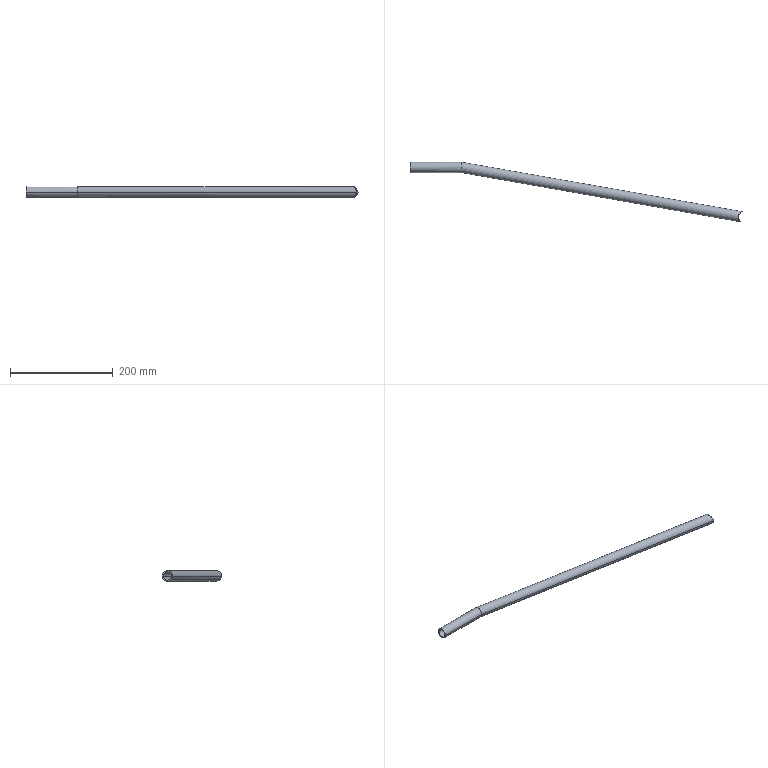Part | SolidWorks | features Cut 1, Sweep 1 | 1 solid | 10 faces | box 645.85 x 115.746 x 20 mm | volume 73442 mm3 | cylinder 9 | plane 1 | commonest cylinder face diameters 16 x4 20 x4 25 x1
STEP:
#1=CARTESIAN_POINT('',(-8.07,9.546,0.));
#2=VERTEX_POINT('',#1);
#3=CARTESIAN_POINT('',(-10.848,-6.211,0.));
#4=VERTEX_POINT('',#3);
#5=CARTESIAN_POINT('',(-8.07,9.546,0.));
#6=CARTESIAN_POINT('',(-8.07,9.546,-0.5418));
#7=CARTESIAN_POINT('',(-8.124,9.501,-1.074));
#8=CARTESIAN_POINT('',(-8.279,9.365,-1.86));
#9=CARTESIAN_POINT('',(-8.343,9.309,-2.12));
#10=CARTESIAN_POINT('',(-8.489,9.176,-2.623));
#11=CARTESIAN_POINT('',(-8.571,9.099,-2.869));
#12=CARTESIAN_POINT('',(-8.842,8.84,-3.586));
#13=CARTESIAN_POINT('',(-9.054,8.625,-4.044));
#14=CARTESIAN_POINT('',(-9.503,8.127,-4.888));
#15=CARTESIAN_POINT('',(-9.742,7.843,-5.28));
#16=CARTESIAN_POINT('',(-10.229,7.196,-6.005));
#17=CARTESIAN_POINT('',(-10.472,6.841,-6.33));
#18=CARTESIAN_POINT('',(-10.822,6.26,-6.76));
#19=CARTESIAN_POINT('',(-10.937,6.058,-6.894));
#20=CARTESIAN_POINT('',(-11.16,5.635,-7.143));
#21=CARTESIAN_POINT('',(-11.269,5.414,-7.258));
#22=CARTESIAN_POINT('',(-11.582,4.728,-7.568));
#23=CARTESIAN_POINT('',(-11.768,4.249,-7.727));
#24=CARTESIAN_POINT('',(-12.005,3.493,-7.889));
#25=CARTESIAN_POINT('',(-12.078,3.233,-7.931));
#26=CARTESIAN_POINT('',(-12.206,2.708,-7.986));
#27=CARTESIAN_POINT('',(-12.262,2.444,-8.));
#28=CARTESIAN_POINT('',(-12.355,1.915,-8.));
#29=CARTESIAN_POINT('',(-12.394,1.65,-7.987));
#30=CARTESIAN_POINT('',(-12.453,1.116,-7.934));
#31=CARTESIAN_POINT('',(-12.474,0.8473,-7.893));
#32=CARTESIAN_POINT('',(-12.511,0.04928,-7.732));
#33=CARTESIAN_POINT('',(-12.501,-0.4657,-7.574));
#34=CARTESIAN_POINT('',(-12.443,-1.214,-7.267));
#35=CARTESIAN_POINT('',(-12.417,-1.461,-7.152));
#36=CARTESIAN_POINT('',(-12.351,-1.938,-6.902));
#37=CARTESIAN_POINT('',(-12.313,-2.169,-6.768));
#38=CARTESIAN_POINT('',(-12.225,-2.616,-6.48));
#39=CARTESIAN_POINT('',(-12.177,-2.832,-6.326));
#40=CARTESIAN_POINT('',(-12.072,-3.251,-6.));
#41=CARTESIAN_POINT('',(-12.015,-3.454,-5.827));
#42=CARTESIAN_POINT('',(-11.838,-4.033,-5.285));
#43=CARTESIAN_POINT('',(-11.712,-4.381,-4.895));
#44=CARTESIAN_POINT('',(-11.46,-5.003,-4.052));
#45=CARTESIAN_POINT('',(-11.334,-5.278,-3.594));
#46=CARTESIAN_POINT('',(-11.113,-5.727,-2.638));
#47=CARTESIAN_POINT('',(-11.019,-5.904,-2.139));
#48=CARTESIAN_POINT('',(-10.885,-6.148,-1.085));
#49=CARTESIAN_POINT('',(-10.848,-6.211,-0.5447));
#50=CARTESIAN_POINT('',(-10.848,-6.211,0.));
#51=B_SPLINE_CURVE_WITH_KNOTS('',3,(#5,#6,#7,#8,#9,#10,#11,#12,#13,#14,#15,#16,#17,#18,#19,#20,#21,#22,#23,#24,#25,#26,#27,#28,#29,#30,#31,#32,#33,#34,#35,#36,#37,#38,#39,#40,#41,#42,#43,#44,#45,#46,#47,#48,#49,#50),.UNSPECIFIED.,.F.,.F.,(4,2,2,2,2,2,2,2,2,2,2,2,2,2,2,2,2,2,2,2,2,2,4),(0.02576,0.02737,0.02817,0.02897,0.03058,0.03218,0.03379,0.03459,0.03539,0.037,0.0378,0.0386,0.0394,0.04021,0.04181,0.04262,0.04342,0.04422,0.04502,0.04663,0.04823,0.04984,0.05144),.UNSPECIFIED.);
#52=EDGE_CURVE('',#2,#4,#51,.T.);
#53=ORIENTED_EDGE('',*,*,#52,.F.);
#54=CARTESIAN_POINT('',(-550.549,105.2,0.));
#55=VERTEX_POINT('',#54);
#56=CARTESIAN_POINT('',(1.389,7.878,0.));
#57=DIRECTION('',(-0.9848,0.1736,0.));
#58=VECTOR('',#57,1000.);
#59=LINE('',#56,#58);
#60=EDGE_CURVE('',#2,#55,#59,.T.);
#61=ORIENTED_EDGE('',*,*,#60,.T.);
#62=CARTESIAN_POINT('',(-551.949,89.2,0.));
#63=VERTEX_POINT('',#62);
#64=CARTESIAN_POINT('',(-550.549,105.2,0.));
#65=CARTESIAN_POINT('',(-550.549,105.2,-16.));
#66=CARTESIAN_POINT('',(-551.949,89.2,-16.));
#67=CARTESIAN_POINT('',(-551.949,89.2,0.));
#68=(BOUNDED_CURVE()B_SPLINE_CURVE(3,(#64,#65,#66,#67),.UNSPECIFIED.,.F.,.T.)B_SPLINE_CURVE_WITH_KNOTS((4,4),(3.142,6.283),.UNSPECIFIED.)CURVE()GEOMETRIC_REPRESENTATION_ITEM()RATIONAL_B_SPLINE_CURVE((1.,0.3333,0.3333,1.))REPRESENTATION_ITEM(''));
#69=EDGE_CURVE('',#55,#63,#68,.T.);
#70=ORIENTED_EDGE('',*,*,#69,.T.);
#71=CARTESIAN_POINT('',(-1.389,-7.878,0.));
#72=DIRECTION('',(-0.9848,0.1736,0.));
#73=VECTOR('',#72,1000.);
#74=LINE('',#71,#73);
#75=EDGE_CURVE('',#4,#63,#74,.T.);
#76=ORIENTED_EDGE('',*,*,#75,.F.);
#77=EDGE_LOOP('',(#53,#61,#70,#76));
#78=FACE_OUTER_BOUND('',#77,.T.);
#79=CARTESIAN_POINT('',(0.,0.,0.));
#80=DIRECTION('',(-0.9848,0.1736,0.));
#81=DIRECTION('',(-0.1736,-0.9848,0.));
#82=AXIS2_PLACEMENT_3D('',#79,#80,#81);
#83=CYLINDRICAL_SURFACE('',#82,8.);
#84=ADVANCED_FACE('',(#78),#83,.F.);
#85=ORIENTED_EDGE('',*,*,#69,.F.);
#86=CARTESIAN_POINT('',(-651.5,105.2,0.));
#87=VERTEX_POINT('',#86);
#88=CARTESIAN_POINT('',(-550.186,105.2,0.));
#89=DIRECTION('',(-1.,0.,0.));
#90=VECTOR('',#89,1000.);
#91=LINE('',#88,#90);
#92=EDGE_CURVE('',#55,#87,#91,.T.);
#93=ORIENTED_EDGE('',*,*,#92,.T.);
#94=CARTESIAN_POINT('',(-651.5,89.2,0.));
#95=VERTEX_POINT('',#94);
#96=CARTESIAN_POINT('',(-651.5,97.2,0.));
#97=DIRECTION('',(1.,0.,0.));
#98=DIRECTION('',(0.,1.,0.));
#99=AXIS2_PLACEMENT_3D('',#96,#97,#98);
#100=CIRCLE('',#99,8.);
#101=EDGE_CURVE('',#95,#87,#100,.T.);
#102=ORIENTED_EDGE('',*,*,#101,.F.);
#103=CARTESIAN_POINT('',(-550.186,89.2,0.));
#104=DIRECTION('',(-1.,0.,0.));
#105=VECTOR('',#104,1000.);
#106=LINE('',#103,#105);
#107=EDGE_CURVE('',#63,#95,#106,.T.);
#108=ORIENTED_EDGE('',*,*,#107,.F.);
#109=EDGE_LOOP('',(#85,#93,#102,#108));
#110=FACE_OUTER_BOUND('',#109,.T.);
#111=CARTESIAN_POINT('',(-550.186,97.2,0.));
#112=DIRECTION('',(-1.,0.,0.));
#113=DIRECTION('',(0.,-1.,0.));
#114=AXIS2_PLACEMENT_3D('',#111,#112,#113);
#115=CYLINDRICAL_SURFACE('',#114,8.);
#116=ADVANCED_FACE('',(#110),#115,.F.);
#117=CARTESIAN_POINT('',(-9.123,-8.546,0.));
#118=VERTEX_POINT('',#117);
#119=CARTESIAN_POINT('',(-5.65,11.15,0.));
#120=VERTEX_POINT('',#119);
#121=CARTESIAN_POINT('',(-9.123,-8.546,0.));
#122=CARTESIAN_POINT('',(-9.123,-8.546,0.7024));
#123=CARTESIAN_POINT('',(-9.208,-8.457,1.382));
#124=CARTESIAN_POINT('',(-9.429,-8.207,2.375));
#125=CARTESIAN_POINT('',(-9.517,-8.105,2.698));
#126=CARTESIAN_POINT('',(-9.711,-7.872,3.32));
#127=CARTESIAN_POINT('',(-9.817,-7.74,3.621));
#128=CARTESIAN_POINT('',(-10.152,-7.302,4.498));
#129=CARTESIAN_POINT('',(-10.4,-6.95,5.055));
#130=CARTESIAN_POINT('',(-10.884,-6.165,6.083));
#131=CARTESIAN_POINT('',(-11.122,-5.729,6.56));
#132=CARTESIAN_POINT('',(-11.567,-4.769,7.445));
#133=CARTESIAN_POINT('',(-11.774,-4.238,7.857));
#134=CARTESIAN_POINT('',(-12.12,-3.113,8.583));
#135=CARTESIAN_POINT('',(-12.261,-2.516,8.9));
#136=CARTESIAN_POINT('',(-12.406,-1.563,9.299));
#137=CARTESIAN_POINT('',(-12.443,-1.235,9.419));
#138=CARTESIAN_POINT('',(-12.491,-0.5751,9.624));
#139=CARTESIAN_POINT('',(-12.502,-0.2411,9.712));
#140=CARTESIAN_POINT('',(-12.497,0.4352,9.853));
#141=CARTESIAN_POINT('',(-12.481,0.7776,9.907));
#142=CARTESIAN_POINT('',(-12.418,1.471,9.981));
#143=CARTESIAN_POINT('',(-12.372,1.815,9.999));
#144=CARTESIAN_POINT('',(-12.253,2.495,10.001));
#145=CARTESIAN_POINT('',(-12.18,2.832,9.983));
#146=CARTESIAN_POINT('',(-12.006,3.498,9.913));
#147=CARTESIAN_POINT('',(-11.904,3.829,9.86));
#148=CARTESIAN_POINT('',(-11.564,4.795,9.649));
#149=CARTESIAN_POINT('',(-11.293,5.398,9.444));
#150=CARTESIAN_POINT('',(-10.831,6.248,9.048));
#151=CARTESIAN_POINT('',(-10.669,6.521,8.901));
#152=CARTESIAN_POINT('',(-10.333,7.04,8.585));
#153=CARTESIAN_POINT('',(-10.16,7.287,8.415));
#154=CARTESIAN_POINT('',(-9.627,7.995,7.871));
#155=CARTESIAN_POINT('',(-9.251,8.423,7.46));
#156=CARTESIAN_POINT('',(-8.502,9.179,6.572));
#157=CARTESIAN_POINT('',(-8.127,9.509,6.094));
#158=CARTESIAN_POINT('',(-7.581,9.942,5.318));
#159=CARTESIAN_POINT('',(-7.401,10.076,5.049));
#160=CARTESIAN_POINT('',(-7.057,10.319,4.497));
#161=CARTESIAN_POINT('',(-6.892,10.43,4.214));
#162=CARTESIAN_POINT('',(-6.582,10.628,3.629));
#163=CARTESIAN_POINT('',(-6.437,10.716,3.328));
#164=CARTESIAN_POINT('',(-6.173,10.87,2.703));
#165=CARTESIAN_POINT('',(-6.054,10.936,2.378));
#166=CARTESIAN_POINT('',(-5.86,11.042,1.719));
#167=CARTESIAN_POINT('',(-5.783,11.082,1.384));
#168=CARTESIAN_POINT('',(-5.677,11.136,0.7));
#169=CARTESIAN_POINT('',(-5.65,11.15,0.3476));
#170=CARTESIAN_POINT('',(-5.65,11.15,0.));
#171=B_SPLINE_CURVE_WITH_KNOTS('',3,(#121,#122,#123,#124,#125,#126,#127,#128,#129,#130,#131,#132,#133,#134,#135,#136,#137,#138,#139,#140,#141,#142,#143,#144,#145,#146,#147,#148,#149,#150,#151,#152,#153,#154,#155,#156,#157,#158,#159,#160,#161,#162,#163,#164,#165,#166,#167,#168,#169,#170),.UNSPECIFIED.,.F.,.F.,(4,2,2,2,2,2,2,2,2,2,2,2,2,2,2,2,2,2,2,2,2,2,2,2,4),(0.,0.002073,0.003109,0.004146,0.006219,0.008292,0.01036,0.01244,0.01347,0.01451,0.01555,0.01658,0.01762,0.01866,0.02073,0.02177,0.0228,0.02487,0.02695,0.02798,0.02902,0.03006,0.03109,0.03213,0.03317),.UNSPECIFIED.);
#172=EDGE_CURVE('',#118,#120,#171,.T.);
#173=ORIENTED_EDGE('',*,*,#172,.T.);
#174=CARTESIAN_POINT('',(-550.374,107.2,0.));
#175=VERTEX_POINT('',#174);
#176=CARTESIAN_POINT('',(1.736,9.848,0.));
#177=DIRECTION('',(-0.9848,0.1736,0.));
#178=VECTOR('',#177,1000.);
#179=LINE('',#176,#178);
#180=EDGE_CURVE('',#120,#175,#179,.T.);
#181=ORIENTED_EDGE('',*,*,#180,.T.);
#182=CARTESIAN_POINT('',(-552.123,87.2,0.));
#183=VERTEX_POINT('',#182);
#184=CARTESIAN_POINT('',(-552.123,87.2,0.));
#185=CARTESIAN_POINT('',(-552.123,87.2,20.));
#186=CARTESIAN_POINT('',(-550.374,107.2,20.));
#187=CARTESIAN_POINT('',(-550.374,107.2,0.));
#188=(BOUNDED_CURVE()B_SPLINE_CURVE(3,(#184,#185,#186,#187),.UNSPECIFIED.,.F.,.F.)B_SPLINE_CURVE_WITH_KNOTS((4,4),(3.142,6.283),.UNSPECIFIED.)CURVE()GEOMETRIC_REPRESENTATION_ITEM()RATIONAL_B_SPLINE_CURVE((1.,0.3333,0.3333,1.))REPRESENTATION_ITEM(''));
#189=EDGE_CURVE('',#183,#175,#188,.T.);
#190=ORIENTED_EDGE('',*,*,#189,.F.);
#191=CARTESIAN_POINT('',(-1.736,-9.848,0.));
#192=DIRECTION('',(-0.9848,0.1736,0.));
#193=VECTOR('',#192,1000.);
#194=LINE('',#191,#193);
#195=EDGE_CURVE('',#118,#183,#194,.T.);
#196=ORIENTED_EDGE('',*,*,#195,.F.);
#197=EDGE_LOOP('',(#173,#181,#190,#196));
#198=FACE_OUTER_BOUND('',#197,.T.);
#199=CARTESIAN_POINT('',(0.,0.,0.));
#200=DIRECTION('',(-0.9848,0.1736,0.));
#201=DIRECTION('',(-0.1736,-0.9848,0.));
#202=AXIS2_PLACEMENT_3D('',#199,#200,#201);
#203=CYLINDRICAL_SURFACE('',#202,10.);
#204=ADVANCED_FACE('',(#198),#203,.T.);
#205=ORIENTED_EDGE('',*,*,#189,.T.);
#206=CARTESIAN_POINT('',(-651.5,107.2,0.));
#207=VERTEX_POINT('',#206);
#208=CARTESIAN_POINT('',(-550.186,107.2,0.));
#209=DIRECTION('',(-1.,0.,0.));
#210=VECTOR('',#209,1000.);
#211=LINE('',#208,#210);
#212=EDGE_CURVE('',#175,#207,#211,.T.);
#213=ORIENTED_EDGE('',*,*,#212,.T.);
#214=CARTESIAN_POINT('',(-651.5,87.2,0.));
#215=VERTEX_POINT('',#214);
#216=CARTESIAN_POINT('',(-651.5,97.2,0.));
#217=DIRECTION('',(1.,0.,0.));
#218=DIRECTION('',(0.,1.,0.));
#219=AXIS2_PLACEMENT_3D('',#216,#217,#218);
#220=CIRCLE('',#219,10.);
#221=EDGE_CURVE('',#207,#215,#220,.T.);
#222=ORIENTED_EDGE('',*,*,#221,.T.);
#223=CARTESIAN_POINT('',(-550.186,87.2,0.));
#224=DIRECTION('',(-1.,0.,0.));
#225=VECTOR('',#224,1000.);
#226=LINE('',#223,#225);
#227=EDGE_CURVE('',#183,#215,#226,.T.);
#228=ORIENTED_EDGE('',*,*,#227,.F.);
#229=EDGE_LOOP('',(#205,#213,#222,#228));
#230=FACE_OUTER_BOUND('',#229,.T.);
#231=CARTESIAN_POINT('',(-550.186,97.2,0.));
#232=DIRECTION('',(-1.,0.,0.));
#233=DIRECTION('',(0.,-1.,0.));
#234=AXIS2_PLACEMENT_3D('',#231,#232,#233);
#235=CYLINDRICAL_SURFACE('',#234,10.);
#236=ADVANCED_FACE('',(#230),#235,.T.);
#237=ORIENTED_EDGE('',*,*,#180,.F.);
#238=CARTESIAN_POINT('',(-5.65,11.15,0.));
#239=CARTESIAN_POINT('',(-5.65,11.15,-0.3473));
#240=CARTESIAN_POINT('',(-5.677,11.137,-0.6913));
#241=CARTESIAN_POINT('',(-5.78,11.083,-1.373));
#242=CARTESIAN_POINT('',(-5.858,11.043,-1.714));
#243=CARTESIAN_POINT('',(-6.151,10.884,-2.704));
#244=CARTESIAN_POINT('',(-6.42,10.732,-3.322));
#245=CARTESIAN_POINT('',(-6.887,10.433,-4.205));
#246=CARTESIAN_POINT('',(-7.054,10.322,-4.492));
#247=CARTESIAN_POINT('',(-7.397,10.079,-5.042));
#248=CARTESIAN_POINT('',(-7.574,9.947,-5.308));
#249=CARTESIAN_POINT('',(-8.114,9.519,-6.077));
#250=CARTESIAN_POINT('',(-8.488,9.192,-6.554));
#251=CARTESIAN_POINT('',(-9.051,8.625,-7.224));
#252=CARTESIAN_POINT('',(-9.24,8.423,-7.438));
#253=CARTESIAN_POINT('',(-9.608,8.001,-7.843));
#254=CARTESIAN_POINT('',(-9.788,7.78,-8.035));
#255=CARTESIAN_POINT('',(-10.317,7.082,-8.575));
#256=CARTESIAN_POINT('',(-10.652,6.573,-8.892));
#257=CARTESIAN_POINT('',(-11.115,5.728,-9.292));
#258=CARTESIAN_POINT('',(-11.263,5.432,-9.412));
#259=CARTESIAN_POINT('',(-11.534,4.829,-9.62));
#260=CARTESIAN_POINT('',(-11.659,4.519,-9.707));
#261=CARTESIAN_POINT('',(-11.887,3.881,-9.85));
#262=CARTESIAN_POINT('',(-11.989,3.554,-9.905));
#263=CARTESIAN_POINT('',(-12.169,2.88,-9.98));
#264=CARTESIAN_POINT('',(-12.244,2.542,-9.999));
#265=CARTESIAN_POINT('',(-12.365,1.862,-10.001));
#266=CARTESIAN_POINT('',(-12.412,1.52,-9.984));
#267=CARTESIAN_POINT('',(-12.477,0.8339,-9.915));
#268=CARTESIAN_POINT('',(-12.495,0.4866,-9.862));
#269=CARTESIAN_POINT('',(-12.507,-0.5377,-9.653));
#270=CARTESIAN_POINT('',(-12.459,-1.198,-9.448));
#271=CARTESIAN_POINT('',(-12.317,-2.156,-9.052));
#272=CARTESIAN_POINT('',(-12.258,-2.469,-8.906));
#273=CARTESIAN_POINT('',(-12.121,-3.072,-8.59));
#274=CARTESIAN_POINT('',(-12.043,-3.364,-8.42));
#275=CARTESIAN_POINT('',(-11.784,-4.212,-7.877));
#276=CARTESIAN_POINT('',(-11.577,-4.744,-7.465));
#277=CARTESIAN_POINT('',(-11.132,-5.712,-6.578));
#278=CARTESIAN_POINT('',(-10.892,-6.151,-6.099));
#279=CARTESIAN_POINT('',(-10.526,-6.746,-5.323));
#280=CARTESIAN_POINT('',(-10.403,-6.934,-5.054));
#281=CARTESIAN_POINT('',(-10.163,-7.281,-4.502));
#282=CARTESIAN_POINT('',(-10.046,-7.441,-4.219));
#283=CARTESIAN_POINT('',(-9.822,-7.734,-3.633));
#284=CARTESIAN_POINT('',(-9.715,-7.867,-3.332));
#285=CARTESIAN_POINT('',(-9.52,-8.102,-2.707));
#286=CARTESIAN_POINT('',(-9.431,-8.205,-2.381));
#287=CARTESIAN_POINT('',(-9.283,-8.371,-1.723));
#288=CARTESIAN_POINT('',(-9.225,-8.436,-1.388));
#289=CARTESIAN_POINT('',(-9.144,-8.523,-0.703));
#290=CARTESIAN_POINT('',(-9.123,-8.546,-0.3509));
#291=CARTESIAN_POINT('',(-9.123,-8.546,0.));
#292=B_SPLINE_CURVE_WITH_KNOTS('',3,(#238,#239,#240,#241,#242,#243,#244,#245,#246,#247,#248,#249,#250,#251,#252,#253,#254,#255,#256,#257,#258,#259,#260,#261,#262,#263,#264,#265,#266,#267,#268,#269,#270,#271,#272,#273,#274,#275,#276,#277,#278,#279,#280,#281,#282,#283,#284,#285,#286,#287,#288,#289,#290,#291),.UNSPECIFIED.,.F.,.F.,(4,2,2,2,2,2,2,2,2,2,2,2,2,2,2,2,2,2,2,2,2,2,2,2,2,2,4),(0.03317,0.0342,0.03524,0.03731,0.03834,0.03938,0.04145,0.04249,0.04352,0.04559,0.04663,0.04767,0.0487,0.04974,0.05077,0.05181,0.05388,0.05492,0.05595,0.05802,0.06009,0.06113,0.06217,0.0632,0.06424,0.06527,0.06631),.UNSPECIFIED.);
#293=EDGE_CURVE('',#120,#118,#292,.T.);
#294=ORIENTED_EDGE('',*,*,#293,.T.);
#295=ORIENTED_EDGE('',*,*,#195,.T.);
#296=CARTESIAN_POINT('',(-550.374,107.2,0.));
#297=CARTESIAN_POINT('',(-550.374,107.2,-20.));
#298=CARTESIAN_POINT('',(-552.123,87.2,-20.));
#299=CARTESIAN_POINT('',(-552.123,87.2,0.));
#300=(BOUNDED_CURVE()B_SPLINE_CURVE(3,(#296,#297,#298,#299),.UNSPECIFIED.,.F.,.F.)B_SPLINE_CURVE_WITH_KNOTS((4,4),(0.,3.142),.UNSPECIFIED.)CURVE()GEOMETRIC_REPRESENTATION_ITEM()RATIONAL_B_SPLINE_CURVE((1.,0.3333,0.3333,1.))REPRESENTATION_ITEM(''));
#301=EDGE_CURVE('',#175,#183,#300,.T.);
#302=ORIENTED_EDGE('',*,*,#301,.F.);
#303=EDGE_LOOP('',(#237,#294,#295,#302));
#304=FACE_OUTER_BOUND('',#303,.T.);
#305=CARTESIAN_POINT('',(0.,0.,0.));
#306=DIRECTION('',(-0.9848,0.1736,0.));
#307=DIRECTION('',(-0.1736,-0.9848,0.));
#308=AXIS2_PLACEMENT_3D('',#305,#306,#307);
#309=CYLINDRICAL_SURFACE('',#308,10.);
#310=ADVANCED_FACE('',(#304),#309,.T.);
#311=ORIENTED_EDGE('',*,*,#212,.F.);
#312=ORIENTED_EDGE('',*,*,#301,.T.);
#313=ORIENTED_EDGE('',*,*,#227,.T.);
#314=CARTESIAN_POINT('',(-651.5,97.2,0.));
#315=DIRECTION('',(1.,0.,0.));
#316=DIRECTION('',(0.,1.,0.));
#317=AXIS2_PLACEMENT_3D('',#314,#315,#316);
#318=CIRCLE('',#317,10.);
#319=EDGE_CURVE('',#215,#207,#318,.T.);
#320=ORIENTED_EDGE('',*,*,#319,.T.);
#321=EDGE_LOOP('',(#311,#312,#313,#320));
#322=FACE_OUTER_BOUND('',#321,.T.);
#323=CARTESIAN_POINT('',(-550.186,97.2,0.));
#324=DIRECTION('',(-1.,0.,0.));
#325=DIRECTION('',(0.,-1.,0.));
#326=AXIS2_PLACEMENT_3D('',#323,#324,#325);
#327=CYLINDRICAL_SURFACE('',#326,10.);
#328=ADVANCED_FACE('',(#322),#327,.T.);
#329=ORIENTED_EDGE('',*,*,#101,.T.);
#330=CARTESIAN_POINT('',(-651.5,97.2,0.));
#331=DIRECTION('',(1.,0.,0.));
#332=DIRECTION('',(0.,1.,0.));
#333=AXIS2_PLACEMENT_3D('',#330,#331,#332);
#334=CIRCLE('',#333,8.);
#335=EDGE_CURVE('',#87,#95,#334,.T.);
#336=ORIENTED_EDGE('',*,*,#335,.T.);
#337=EDGE_LOOP('',(#329,#336));
#338=FACE_BOUND('',#337,.T.);
#339=ORIENTED_EDGE('',*,*,#319,.F.);
#340=ORIENTED_EDGE('',*,*,#221,.F.);
#341=EDGE_LOOP('',(#339,#340));
#342=FACE_OUTER_BOUND('',#341,.T.);
#343=CARTESIAN_POINT('',(-651.5,97.2,0.));
#344=DIRECTION('',(1.,0.,0.));
#345=DIRECTION('',(0.,1.,0.));
#346=AXIS2_PLACEMENT_3D('',#343,#344,#345);
#347=PLANE('',#346);
#348=ADVANCED_FACE('',(#338,#342),#347,.F.);
#349=ORIENTED_EDGE('',*,*,#60,.F.);
#350=CARTESIAN_POINT('',(-10.848,-6.211,0.));
#351=CARTESIAN_POINT('',(-10.848,-6.211,0.5463));
#352=CARTESIAN_POINT('',(-10.884,-6.148,1.079));
#353=CARTESIAN_POINT('',(-11.016,-5.909,2.12));
#354=CARTESIAN_POINT('',(-11.112,-5.73,2.631));
#355=CARTESIAN_POINT('',(-11.332,-5.282,3.587));
#356=CARTESIAN_POINT('',(-11.457,-5.011,4.04));
#357=CARTESIAN_POINT('',(-11.711,-4.385,4.891));
#358=CARTESIAN_POINT('',(-11.837,-4.036,5.282));
#359=CARTESIAN_POINT('',(-12.072,-3.268,6.001));
#360=CARTESIAN_POINT('',(-12.181,-2.844,6.332));
#361=CARTESIAN_POINT('',(-12.355,-1.952,6.908));
#362=CARTESIAN_POINT('',(-12.422,-1.482,7.155));
#363=CARTESIAN_POINT('',(-12.5,-0.4904,7.565));
#364=CARTESIAN_POINT('',(-12.511,0.03642,7.728));
#365=CARTESIAN_POINT('',(-12.464,1.087,7.943));
#366=CARTESIAN_POINT('',(-12.407,1.617,7.999));
#367=CARTESIAN_POINT('',(-12.267,2.42,8.001));
#368=CARTESIAN_POINT('',(-12.211,2.688,7.987));
#369=CARTESIAN_POINT('',(-12.084,3.21,7.934));
#370=CARTESIAN_POINT('',(-12.013,3.467,7.894));
#371=CARTESIAN_POINT('',(-11.777,4.223,7.734));
#372=CARTESIAN_POINT('',(-11.588,4.714,7.573));
#373=CARTESIAN_POINT('',(-11.174,5.625,7.164));
#374=CARTESIAN_POINT('',(-10.949,6.049,6.915));
#375=CARTESIAN_POINT('',(-10.474,6.838,6.333));
#376=CARTESIAN_POINT('',(-10.23,7.194,6.007));
#377=CARTESIAN_POINT('',(-9.868,7.676,5.467));
#378=CARTESIAN_POINT('',(-9.747,7.828,5.279));
#379=CARTESIAN_POINT('',(-9.509,8.116,4.884));
#380=CARTESIAN_POINT('',(-9.392,8.251,4.678));
#381=CARTESIAN_POINT('',(-9.054,8.625,4.044));
#382=CARTESIAN_POINT('',(-8.846,8.835,3.596));
#383=CARTESIAN_POINT('',(-8.486,9.182,2.642));
#384=CARTESIAN_POINT('',(-8.333,9.318,2.13));
#385=CARTESIAN_POINT('',(-8.178,9.454,1.347));
#386=CARTESIAN_POINT('',(-8.138,9.488,1.082));
#387=CARTESIAN_POINT('',(-8.084,9.534,0.5459));
#388=CARTESIAN_POINT('',(-8.07,9.546,0.2717));
#389=CARTESIAN_POINT('',(-8.07,9.546,0.));
#390=B_SPLINE_CURVE_WITH_KNOTS('',3,(#350,#351,#352,#353,#354,#355,#356,#357,#358,#359,#360,#361,#362,#363,#364,#365,#366,#367,#368,#369,#370,#371,#372,#373,#374,#375,#376,#377,#378,#379,#380,#381,#382,#383,#384,#385,#386,#387,#388,#389),.UNSPECIFIED.,.F.,.F.,(4,2,2,2,2,2,2,2,2,2,2,2,2,2,2,2,2,2,2,4),(0.,0.00161,0.00322,0.00483,0.00644,0.00805,0.00966,0.01127,0.01288,0.01369,0.01449,0.0161,0.01771,0.01932,0.02013,0.02093,0.02254,0.02415,0.02496,0.02576),.UNSPECIFIED.);
#391=EDGE_CURVE('',#4,#2,#390,.T.);
#392=ORIENTED_EDGE('',*,*,#391,.F.);
#393=ORIENTED_EDGE('',*,*,#75,.T.);
#394=CARTESIAN_POINT('',(-551.949,89.2,0.));
#395=CARTESIAN_POINT('',(-551.949,89.2,16.));
#396=CARTESIAN_POINT('',(-550.549,105.2,16.));
#397=CARTESIAN_POINT('',(-550.549,105.2,0.));
#398=(BOUNDED_CURVE()B_SPLINE_CURVE(3,(#394,#395,#396,#397),.UNSPECIFIED.,.F.,.F.)B_SPLINE_CURVE_WITH_KNOTS((4,4),(0.,3.142),.UNSPECIFIED.)CURVE()GEOMETRIC_REPRESENTATION_ITEM()RATIONAL_B_SPLINE_CURVE((1.,0.3333,0.3333,1.))REPRESENTATION_ITEM(''));
#399=EDGE_CURVE('',#63,#55,#398,.T.);
#400=ORIENTED_EDGE('',*,*,#399,.T.);
#401=EDGE_LOOP('',(#349,#392,#393,#400));
#402=FACE_OUTER_BOUND('',#401,.T.);
#403=CARTESIAN_POINT('',(0.,0.,0.));
#404=DIRECTION('',(-0.9848,0.1736,0.));
#405=DIRECTION('',(-0.1736,-0.9848,0.));
#406=AXIS2_PLACEMENT_3D('',#403,#404,#405);
#407=CYLINDRICAL_SURFACE('',#406,8.);
#408=ADVANCED_FACE('',(#402),#407,.F.);
#409=ORIENTED_EDGE('',*,*,#92,.F.);
#410=ORIENTED_EDGE('',*,*,#399,.F.);
#411=ORIENTED_EDGE('',*,*,#107,.T.);
#412=ORIENTED_EDGE('',*,*,#335,.F.);
#413=EDGE_LOOP('',(#409,#410,#411,#412));
#414=FACE_OUTER_BOUND('',#413,.T.);
#415=CARTESIAN_POINT('',(-550.186,97.2,0.));
#416=DIRECTION('',(-1.,0.,0.));
#417=DIRECTION('',(0.,-1.,0.));
#418=AXIS2_PLACEMENT_3D('',#415,#416,#417);
#419=CYLINDRICAL_SURFACE('',#418,8.);
#420=ADVANCED_FACE('',(#414),#419,.F.);
#421=ORIENTED_EDGE('',*,*,#391,.T.);
#422=ORIENTED_EDGE('',*,*,#52,.T.);
#423=EDGE_LOOP('',(#421,#422));
#424=FACE_BOUND('',#423,.T.);
#425=ORIENTED_EDGE('',*,*,#172,.F.);
#426=ORIENTED_EDGE('',*,*,#293,.F.);
#427=EDGE_LOOP('',(#425,#426));
#428=FACE_OUTER_BOUND('',#427,.T.);
#429=CARTESIAN_POINT('',(0.,0.,-10.));
#430=DIRECTION('',(0.,0.,1.));
#431=DIRECTION('',(1.,0.,0.));
#432=AXIS2_PLACEMENT_3D('',#429,#430,#431);
#433=CYLINDRICAL_SURFACE('',#432,12.5);
#434=ADVANCED_FACE('',(#424,#428),#433,.F.);
#435=CLOSED_SHELL('',(#84,#116,#204,#236,#310,#328,#348,#408,#420,#434));
#436=MANIFOLD_SOLID_BREP('',#435);
#437=CARTESIAN_POINT('',(0.,0.,0.));
#438=DIRECTION('',(0.,0.,1.));
#439=DIRECTION('',(1.,0.,0.));
#440=AXIS2_PLACEMENT_3D('',#437,#438,#439);
#441=(LENGTH_UNIT()NAMED_UNIT(*)SI_UNIT(.MILLI.,.METRE.));
#442=UNCERTAINTY_MEASURE_WITH_UNIT(LENGTH_MEASURE(0.00001),#441,'','');
#443=(NAMED_UNIT(*)PLANE_ANGLE_UNIT()SI_UNIT($,.RADIAN.));
#444=(NAMED_UNIT(*)SI_UNIT($,.STERADIAN.)SOLID_ANGLE_UNIT());
#445=(GEOMETRIC_REPRESENTATION_CONTEXT(3)GLOBAL_UNCERTAINTY_ASSIGNED_CONTEXT((#442))GLOBAL_UNIT_ASSIGNED_CONTEXT((#441,#443,#444))REPRESENTATION_CONTEXT('',''));
#446=ADVANCED_BREP_SHAPE_REPRESENTATION('',(#436,#440),#445);